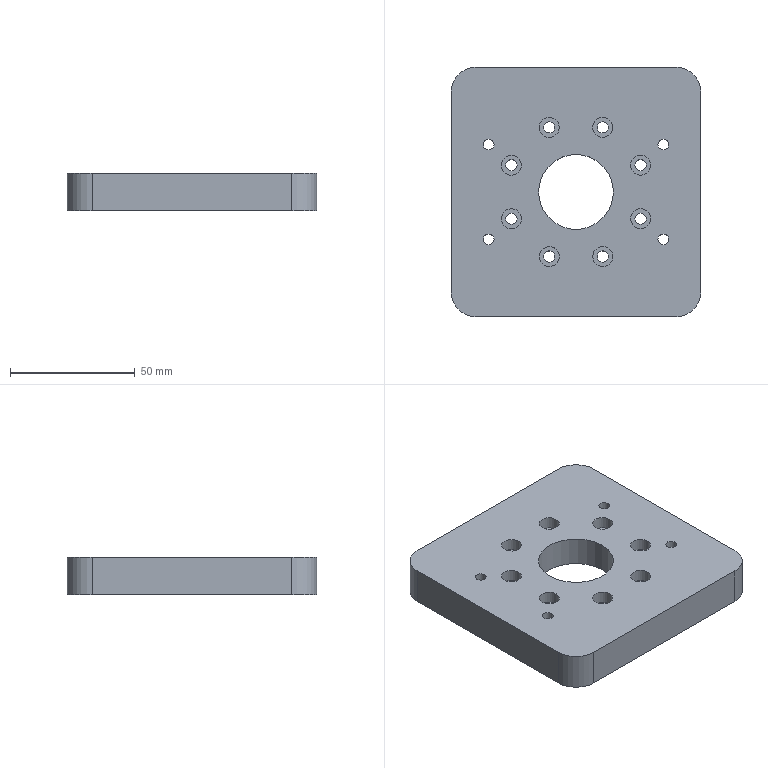NC program | NX | posted with a generic post | part box 100 x 100 x 15 mm
Whole program:
N10 G17 G21 G94 G90
(FLOOR_WALL_1_COPY , TOOL : D63)
N12 T01 M6
N14 G54
N16 G17 G0 G90 X-84.5 Y49.997 S6500 M3
N18 G43 Z30. H1
N20 Z5.
N22 G94 G1 Z2. F1500.
N24 X-81.5
N26 X81.5
N28 Y25.065
N30 X-81.5
N32 Y0.132
N34 X81.5
N36 Y-24.8
N38 X-81.5
N40 X-84.5
N42 Z5.
N44 G0 Z30.
N46 Y49.997
N48 Z4.
N50 G1 Z1.
N52 X-81.5
N54 X81.5
N56 Y25.065
N58 X-81.5
N60 Y0.132
N62 X81.5
N64 Y-24.8
N66 X-81.5
N68 X-84.5
N70 Z4.
N72 G0 Z30.
N74 Y49.997
N76 Z3.
N78 G1 Z0.
N80 X-81.5
N82 X81.5
N84 Y25.065
N86 X-81.5
N88 Y0.132
N90 X81.5
N92 Y-24.8
N94 X-81.5
N96 X-84.5
N98 Z3.
N100 G0 Z30.
N102 M5
(HOLE_MILLING_COPY_1 , TOOL : D10)
N104 T10 M6
N106 G54
N108 G17 G0 G90 X0. Y0. S9500 M3
N110 G43 Z30. H10
N112 Z0.5
N114 G94 G1 X-0.831 Y1.819 F2200.
N116 G3 X-9.19 Y0. R4.377
N118 X-9.19 Y0. Z-0.5 I9.19 J0.
N120 X-9.19 Y0. Z-1.5 I9.19 J0.
N122 X-9.19 Y0. Z-2.5 I9.19 J0.
N124 X9.19 Y0. Z-3. I9.19 J0.
N126 X0. Y9.19 R9.19
N128 X9.19 Y0. R-9.19
N130 X0.831 Y1.819 R4.377
N132 G1 X0. Y0.
N134 G0 Z0.5
N136 G1 X-0.585 Y1.913
N138 G3 X-13.38 Y0. R6.541
N140 X-13.38 Y0. Z-0.5 I13.38 J0.
N142 X-13.38 Y0. Z-1.5 I13.38 J0.
N144 X-13.38 Y0. Z-2.5 I13.38 J0.
N146 X13.38 Y0. Z-3. I13.38 J0.
N148 X0. Y13.38 R13.38
N150 X13.38 Y0. R-13.38
N152 X0.585 Y1.913 R6.541
N154 G1 X0. Y0.
N156 G0 Z0.5
N158 G1 X-0.449 Y1.949
N160 G3 X-17.57 Y0. R8.671
N162 X-17.57 Y0. Z-0.5 I17.57 J0.
N164 X-17.57 Y0. Z-1.5 I17.57 J0.
N166 X-17.57 Y0. Z-2.5 I17.57 J0.
N168 X17.57 Y0. Z-3. I17.57 J0.
N170 X0. Y17.57 R17.57
N172 X17.57 Y0. R-17.57
N174 X0.449 Y1.949 R8.671
N176 G1 X0. Y0.
N178 G0 Z0.5
N180 G1 X-0.365 Y1.966
N182 G3 X-21.76 Y0. R10.788
N184 X-21.76 Y0. Z-0.5 I21.76 J0.
N186 X-21.76 Y0. Z-1.5 I21.76 J0.
N188 X-21.76 Y0. Z-2.5 I21.76 J0.
N190 X21.76 Y0. Z-3. I21.76 J0.
N192 X0. Y21.76 R21.76
N194 X21.76 Y0. R-21.76
N196 X0.365 Y1.966 R10.788
N198 G1 X0. Y0.
N200 G0 Z0.5
N202 G1 X-0.306 Y1.976
N204 G3 X-25.95 Y0. R12.898
N206 X-25.95 Y0. Z-0.5 I25.95 J0.
N208 X-25.95 Y0. Z-1.5 I25.95 J0.
N210 X-25.95 Y0. Z-2.5 I25.95 J0.
N212 X25.95 Y0. Z-3. I25.95 J0.
N214 X0. Y25.95 R25.95
N216 X25.95 Y0. R-25.95
N218 X0.306 Y1.976 R12.898
N220 G1 X0. Y0.
N222 G0 Z30.
(10 , TOOL : D10)
N224 X-22.767 Y2.892
N226 Z0.5
N228 G3 X-26.05 Y0. R2.916 F1200.
N230 X-26.05 Y0. Z-2.5 I26.05 J0.
N232 X-13.025 Y-22.56 Z-3. R26.05
N234 X22.56 Y-13.025 R26.05
N236 X-13.025 Y-22.56 R-26.05
N238 X-8.879 Y-21.163 R2.916
N240 G0 Z30.
N242 M5
(PLANAR_MILL_COPY , TOOL : D6A45)
N244 T07 M6
N246 G54
N248 G17 G0 G90 X35.75 Y-19.866 S9500 M3
N250 G43 Z30. H7
N252 Z0.5
N254 G94 G1 Z-1. F1250.
N256 G3 X36.25 Y-19. R1.
N258 X35. Y-17.75 R1.25
N260 X36.25 Y-19. R-1.25
N262 X35.75 Y-18.134 R1.
N264 G1 Z0.5
N266 G0 Z30.
N268 Y18.134
N270 Z0.5
N272 G1 Z-1.
N274 G3 X36.25 Y19. R1.
N276 X35. Y20.25 R1.25
N278 X36.25 Y19. R-1.25
N280 X35.75 Y19.866 R1.
N282 G1 Z0.5
N284 G0 Z30.
N286 X29.65 Y-0.866
N288 Z0.5
N290 G1 Z-1.
N292 G3 X30.15 Y0. R1.
N294 X0. Y30.15 R30.15
N296 X30.15 Y0. R-30.15
N298 X29.65 Y0.866 R1.
N300 G1 Z0.5
N302 G0 Z30.
N304 X51.4
N306 Z0.5
N308 G1 Z-1.
N310 G3 X50.9 Y0. R1.
N312 G1 Y-40.
N314 G2 X40. Y-50.9 R10.9
N316 G1 X-40.
N318 G2 X-50.9 Y-40. R10.9
N320 G1 Y40.
N322 G2 X-40. Y50.9 R10.9
N324 G1 X40.
N326 G2 X50.9 Y40. R10.9
N328 G1 Y0.
N330 G3 X51.4 Y-0.866 R1.
N332 G1 Z0.5
N334 G0 Z30.
N336 X-35.75 Y-18.134
N338 Z0.5
N340 G1 Z-1.
N342 G3 X-36.25 Y-19. R1.
N344 X-35. Y-20.25 R1.25
N346 X-36.25 Y-19. R-1.25
N348 X-35.75 Y-19.866 R1.
N350 G1 Z0.5
N352 G0 Z30.
N354 Y19.866
N356 Z0.5
N358 G1 Z-1.
N360 G3 X-36.25 Y19. R1.
N362 X-35. Y17.75 R1.25
N364 X-36.25 Y19. R-1.25
N366 X-35.75 Y18.134 R1.
N368 G1 Z0.5
N370 G0 Z30.
(PLANAR_MILL_COPY_COPY , TOOL : D6A45)
N372 X-13.6 Y0.866
N374 Z-2.5
N376 G1 Z-4.
N378 G3 X-14.1 Y0. R1.
N380 X0. Y-14.1 R14.1
N382 X-14.1 Y0. R-14.1
N384 X-13.6 Y-0.866 R1.
N386 G1 Z-2.5
N388 G0 Z30.
N390 M5
N392 M2